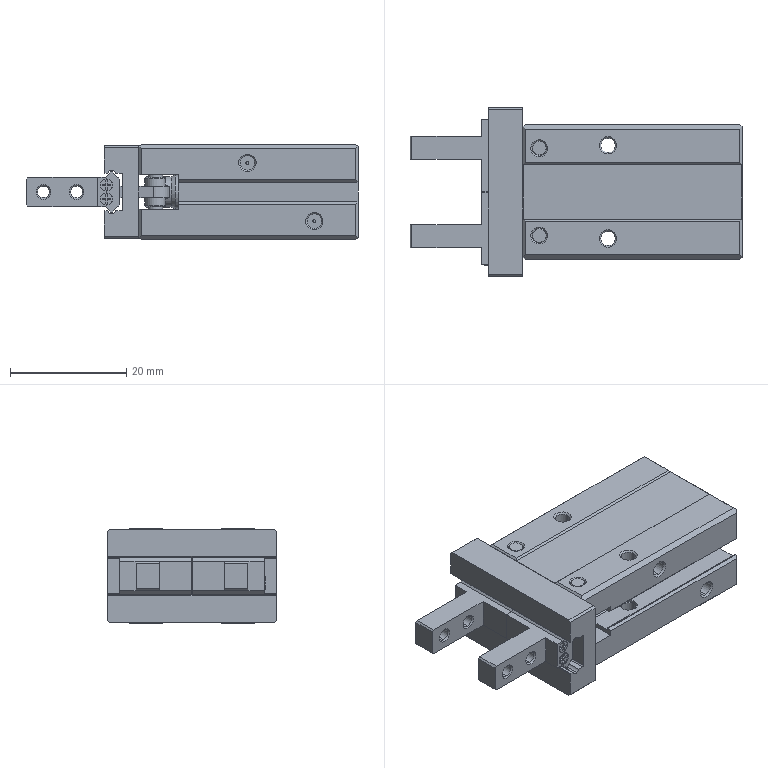Part | STEP file | HFZ10_CL_ | 1 solid | 427 faces | box 57 x 29 x 16.4 mm | volume 14372 mm3 | plane 216 | cylinder 136 | cone 67 | torus 8 | commonest cylinder face diameters 2.459 x20 0.4 x14 2 x10 0.27 x8 2.013 x8 2.1 x8